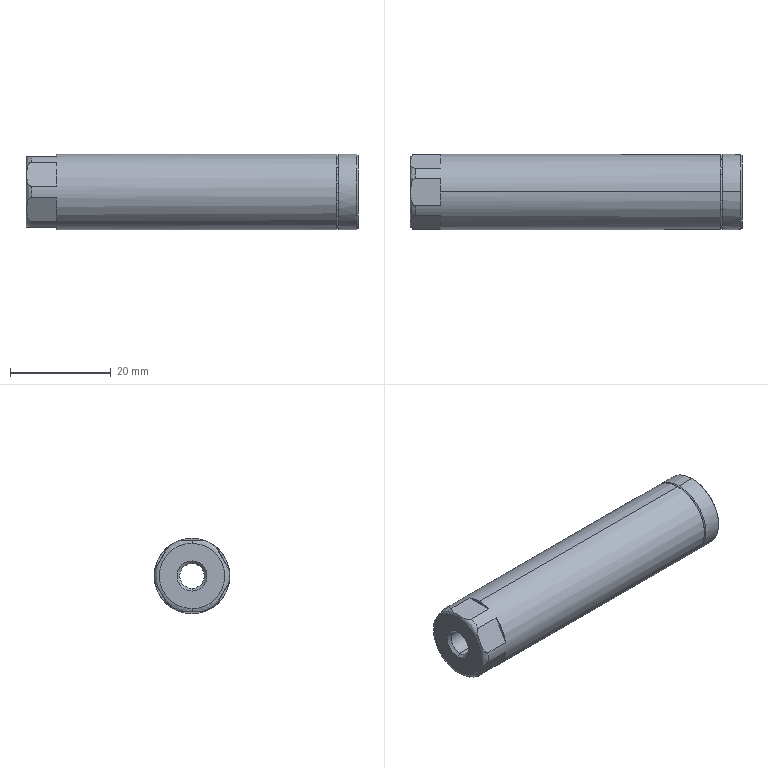Part | SolidWorks | features BaseBody 1 | 1 solid | 34 faces | box 66 x 15 x 15 mm | volume 8114 mm3 | plane 14 | cone 10 | cylinder 8 | spline 2 | commonest cylinder face diameters 15 x4 4.917 x2 8.5 x2
STEP:
#1=CARTESIAN_POINT('',(1.,-2.693,7.));
#2=VERTEX_POINT('',#1);
#3=CARTESIAN_POINT('',(0.134,0.,7.));
#4=VERTEX_POINT('',#3);
#5=CARTESIAN_POINT('',(1.,-2.693,7.));
#6=CARTESIAN_POINT('',(0.9357,-2.693,7.));
#7=CARTESIAN_POINT('',(0.8731,-2.675,7.));
#8=CARTESIAN_POINT('',(0.7611,-2.616,7.));
#9=CARTESIAN_POINT('',(0.7108,-2.575,7.));
#10=CARTESIAN_POINT('',(0.5795,-2.438,7.));
#11=CARTESIAN_POINT('',(0.5135,-2.327,7.));
#12=CARTESIAN_POINT('',(0.4066,-2.1,7.));
#13=CARTESIAN_POINT('',(0.3648,-1.98,7.));
#14=CARTESIAN_POINT('',(0.2958,-1.738,7.));
#15=CARTESIAN_POINT('',(0.2688,-1.616,7.));
#16=CARTESIAN_POINT('',(0.2018,-1.247,7.));
#17=CARTESIAN_POINT('',(0.1754,-0.9993,7.));
#18=CARTESIAN_POINT('',(0.1414,-0.5011,7.));
#19=CARTESIAN_POINT('',(0.134,-0.2503,7.));
#20=CARTESIAN_POINT('',(0.134,0.,7.));
#21=B_SPLINE_CURVE_WITH_KNOTS('',3,(#5,#6,#7,#8,#9,#10,#11,#12,#13,#14,#15,#16,#17,#18,#19,#20),.UNSPECIFIED.,.F.,.F.,(4,2,2,2,2,2,2,4),(0.,0.0001898,0.0003795,0.0007591,0.001139,0.001518,0.002277,0.003036),.UNSPECIFIED.);
#22=EDGE_CURVE('',#2,#4,#21,.T.);
#23=ORIENTED_EDGE('',*,*,#22,.T.);
#24=CARTESIAN_POINT('',(0.,0.,6.5));
#25=VERTEX_POINT('',#24);
#26=CARTESIAN_POINT('',(1.,0.,6.5));
#27=DIRECTION('',(0.,-1.,0.));
#28=DIRECTION('',(0.,0.,1.));
#29=AXIS2_PLACEMENT_3D('',#26,#27,#28);
#30=CIRCLE('',#29,1.);
#31=EDGE_CURVE('',#4,#25,#30,.T.);
#32=ORIENTED_EDGE('',*,*,#31,.T.);
#33=CARTESIAN_POINT('',(0.,0.,-6.5));
#34=VERTEX_POINT('',#33);
#35=CARTESIAN_POINT('',(0.,0.,6.5));
#36=CARTESIAN_POINT('',(0.,-13.,6.5));
#37=CARTESIAN_POINT('',(0.,-13.,-6.5));
#38=CARTESIAN_POINT('',(0.,0.,-6.5));
#39=(BOUNDED_CURVE()B_SPLINE_CURVE(3,(#35,#36,#37,#38),.UNSPECIFIED.,.F.,.F.)B_SPLINE_CURVE_WITH_KNOTS((4,4),(0.5,1.),.UNSPECIFIED.)CURVE()GEOMETRIC_REPRESENTATION_ITEM()RATIONAL_B_SPLINE_CURVE((1.,0.3333,0.3333,1.))REPRESENTATION_ITEM(''));
#40=EDGE_CURVE('',#25,#34,#39,.T.);
#41=ORIENTED_EDGE('',*,*,#40,.T.);
#42=CARTESIAN_POINT('',(0.134,0.,-7.));
#43=VERTEX_POINT('',#42);
#44=CARTESIAN_POINT('',(1.,0.,-6.5));
#45=DIRECTION('',(0.,1.,0.));
#46=DIRECTION('',(0.,0.,-1.));
#47=AXIS2_PLACEMENT_3D('',#44,#45,#46);
#48=CIRCLE('',#47,1.);
#49=EDGE_CURVE('',#43,#34,#48,.T.);
#50=ORIENTED_EDGE('',*,*,#49,.F.);
#51=CARTESIAN_POINT('',(1.,-2.693,-7.));
#52=VERTEX_POINT('',#51);
#53=CARTESIAN_POINT('',(0.134,0.,-7.));
#54=CARTESIAN_POINT('',(0.134,-0.2506,-7.));
#55=CARTESIAN_POINT('',(0.1413,-0.5008,-7.));
#56=CARTESIAN_POINT('',(0.1755,-0.9999,-7.));
#57=CARTESIAN_POINT('',(0.2019,-1.249,-7.));
#58=CARTESIAN_POINT('',(0.2924,-1.744,-7.));
#59=CARTESIAN_POINT('',(0.3546,-1.991,-7.));
#60=CARTESIAN_POINT('',(0.515,-2.33,-7.));
#61=CARTESIAN_POINT('',(0.5805,-2.44,-7.));
#62=CARTESIAN_POINT('',(0.7127,-2.576,-7.));
#63=CARTESIAN_POINT('',(0.7616,-2.616,-7.));
#64=CARTESIAN_POINT('',(0.8736,-2.675,-7.));
#65=CARTESIAN_POINT('',(0.9361,-2.693,-7.));
#66=CARTESIAN_POINT('',(1.,-2.693,-7.));
#67=B_SPLINE_CURVE_WITH_KNOTS('',3,(#53,#54,#55,#56,#57,#58,#59,#60,#61,#62,#63,#64,#65,#66),.UNSPECIFIED.,.F.,.F.,(4,2,2,2,2,2,4),(0.003036,0.003796,0.004556,0.005316,0.005696,0.005886,0.006076),.UNSPECIFIED.);
#68=EDGE_CURVE('',#43,#52,#67,.T.);
#69=ORIENTED_EDGE('',*,*,#68,.T.);
#70=CARTESIAN_POINT('',(1.,-4.716,-5.832));
#71=VERTEX_POINT('',#70);
#72=CARTESIAN_POINT('',(1.,0.,0.));
#73=DIRECTION('',(1.,0.,0.));
#74=DIRECTION('',(0.,0.,1.));
#75=AXIS2_PLACEMENT_3D('',#72,#73,#74);
#76=CIRCLE('',#75,7.5);
#77=EDGE_CURVE('',#71,#52,#76,.T.);
#78=ORIENTED_EDGE('',*,*,#77,.F.);
#79=CARTESIAN_POINT('',(1.,-7.408,-1.168));
#80=VERTEX_POINT('',#79);
#81=CARTESIAN_POINT('',(1.,-4.716,-5.832));
#82=CARTESIAN_POINT('',(0.9356,-4.716,-5.832));
#83=CARTESIAN_POINT('',(0.873,-4.725,-5.816));
#84=CARTESIAN_POINT('',(0.7609,-4.754,-5.765));
#85=CARTESIAN_POINT('',(0.7107,-4.775,-5.73));
#86=CARTESIAN_POINT('',(0.5793,-4.843,-5.611));
#87=CARTESIAN_POINT('',(0.5133,-4.899,-5.515));
#88=CARTESIAN_POINT('',(0.4064,-5.012,-5.318));
#89=CARTESIAN_POINT('',(0.3646,-5.072,-5.214));
#90=CARTESIAN_POINT('',(0.2956,-5.194,-5.004));
#91=CARTESIAN_POINT('',(0.2686,-5.255,-4.898));
#92=CARTESIAN_POINT('',(0.2016,-5.439,-4.579));
#93=CARTESIAN_POINT('',(0.1753,-5.563,-4.364));
#94=CARTESIAN_POINT('',(0.1413,-5.812,-3.933));
#95=CARTESIAN_POINT('',(0.1339,-5.938,-3.715));
#96=CARTESIAN_POINT('',(0.134,-6.188,-3.282));
#97=CARTESIAN_POINT('',(0.1414,-6.313,-3.065));
#98=CARTESIAN_POINT('',(0.1756,-6.563,-2.633));
#99=CARTESIAN_POINT('',(0.2021,-6.687,-2.417));
#100=CARTESIAN_POINT('',(0.2926,-6.935,-1.989));
#101=CARTESIAN_POINT('',(0.3548,-7.058,-1.776));
#102=CARTESIAN_POINT('',(0.5151,-7.227,-1.482));
#103=CARTESIAN_POINT('',(0.5807,-7.282,-1.387));
#104=CARTESIAN_POINT('',(0.7128,-7.35,-1.269));
#105=CARTESIAN_POINT('',(0.7617,-7.37,-1.234));
#106=CARTESIAN_POINT('',(0.8737,-7.4,-1.183));
#107=CARTESIAN_POINT('',(0.9361,-7.408,-1.168));
#108=CARTESIAN_POINT('',(1.,-7.408,-1.168));
#109=B_SPLINE_CURVE_WITH_KNOTS('',3,(#81,#82,#83,#84,#85,#86,#87,#88,#89,#90,#91,#92,#93,#94,#95,#96,#97,#98,#99,#100,#101,#102,#103,#104,#105,#106,#107,#108),.UNSPECIFIED.,.F.,.F.,(4,2,2,2,2,2,2,2,2,2,2,2,2,4),(0.,0.0001899,0.0003798,0.0007595,0.001139,0.001519,0.002279,0.003038,0.003798,0.004557,0.005317,0.005697,0.005887,0.006076),.UNSPECIFIED.);
#110=EDGE_CURVE('',#71,#80,#109,.T.);
#111=ORIENTED_EDGE('',*,*,#110,.T.);
#112=CARTESIAN_POINT('',(1.,-7.408,1.168));
#113=VERTEX_POINT('',#112);
#114=CARTESIAN_POINT('',(1.,0.,0.));
#115=DIRECTION('',(1.,0.,0.));
#116=DIRECTION('',(0.,0.,1.));
#117=AXIS2_PLACEMENT_3D('',#114,#115,#116);
#118=CIRCLE('',#117,7.5);
#119=EDGE_CURVE('',#113,#80,#118,.T.);
#120=ORIENTED_EDGE('',*,*,#119,.F.);
#121=CARTESIAN_POINT('',(1.,-4.716,5.832));
#122=VERTEX_POINT('',#121);
#123=CARTESIAN_POINT('',(1.,-7.408,1.168));
#124=CARTESIAN_POINT('',(0.9356,-7.408,1.168));
#125=CARTESIAN_POINT('',(0.873,-7.4,1.184));
#126=CARTESIAN_POINT('',(0.7609,-7.37,1.235));
#127=CARTESIAN_POINT('',(0.7107,-7.35,1.27));
#128=CARTESIAN_POINT('',(0.5793,-7.281,1.389));
#129=CARTESIAN_POINT('',(0.5133,-7.226,1.485));
#130=CARTESIAN_POINT('',(0.4064,-7.112,1.682));
#131=CARTESIAN_POINT('',(0.3646,-7.052,1.786));
#132=CARTESIAN_POINT('',(0.2956,-6.931,1.996));
#133=CARTESIAN_POINT('',(0.2686,-6.87,2.102));
#134=CARTESIAN_POINT('',(0.2016,-6.685,2.421));
#135=CARTESIAN_POINT('',(0.1753,-6.561,2.636));
#136=CARTESIAN_POINT('',(0.1413,-6.312,3.067));
#137=CARTESIAN_POINT('',(0.1339,-6.187,3.285));
#138=CARTESIAN_POINT('',(0.134,-5.936,3.718));
#139=CARTESIAN_POINT('',(0.1414,-5.811,3.935));
#140=CARTESIAN_POINT('',(0.1756,-5.562,4.367));
#141=CARTESIAN_POINT('',(0.2021,-5.437,4.583));
#142=CARTESIAN_POINT('',(0.2926,-5.19,5.011));
#143=CARTESIAN_POINT('',(0.3548,-5.067,5.224));
#144=CARTESIAN_POINT('',(0.5151,-4.897,5.518));
#145=CARTESIAN_POINT('',(0.5807,-4.842,5.613));
#146=CARTESIAN_POINT('',(0.7128,-4.774,5.731));
#147=CARTESIAN_POINT('',(0.7617,-4.754,5.766));
#148=CARTESIAN_POINT('',(0.8737,-4.725,5.817));
#149=CARTESIAN_POINT('',(0.9361,-4.716,5.832));
#150=CARTESIAN_POINT('',(1.,-4.716,5.832));
#151=B_SPLINE_CURVE_WITH_KNOTS('',3,(#123,#124,#125,#126,#127,#128,#129,#130,#131,#132,#133,#134,#135,#136,#137,#138,#139,#140,#141,#142,#143,#144,#145,#146,#147,#148,#149,#150),.UNSPECIFIED.,.F.,.F.,(4,2,2,2,2,2,2,2,2,2,2,2,2,4),(0.,0.0001899,0.0003798,0.0007595,0.001139,0.001519,0.002279,0.003038,0.003798,0.004557,0.005317,0.005697,0.005887,0.006076),.UNSPECIFIED.);
#152=EDGE_CURVE('',#113,#122,#151,.T.);
#153=ORIENTED_EDGE('',*,*,#152,.T.);
#154=CARTESIAN_POINT('',(1.,0.,0.));
#155=DIRECTION('',(1.,0.,0.));
#156=DIRECTION('',(0.,0.,1.));
#157=AXIS2_PLACEMENT_3D('',#154,#155,#156);
#158=CIRCLE('',#157,7.5);
#159=EDGE_CURVE('',#2,#122,#158,.T.);
#160=ORIENTED_EDGE('',*,*,#159,.F.);
#161=EDGE_LOOP('',(#23,#32,#41,#50,#69,#78,#111,#120,#153,#160));
#162=FACE_OUTER_BOUND('',#161,.T.);
#163=CARTESIAN_POINT('',(1.,0.,7.5));
#164=CARTESIAN_POINT('',(1.,-15.,7.5));
#165=CARTESIAN_POINT('',(1.,-15.,-7.5));
#166=CARTESIAN_POINT('',(1.,0.,-7.5));
#167=CARTESIAN_POINT('',(0.4142,0.,7.5));
#168=CARTESIAN_POINT('',(0.4142,-15.,7.5));
#169=CARTESIAN_POINT('',(0.4142,-15.,-7.5));
#170=CARTESIAN_POINT('',(0.4142,0.,-7.5));
#171=CARTESIAN_POINT('',(0.,0.,7.086));
#172=CARTESIAN_POINT('',(0.,-14.172,7.086));
#173=CARTESIAN_POINT('',(0.,-14.172,-7.086));
#174=CARTESIAN_POINT('',(0.,0.,-7.086));
#175=CARTESIAN_POINT('',(0.,0.,6.5));
#176=CARTESIAN_POINT('',(0.,-13.,6.5));
#177=CARTESIAN_POINT('',(0.,-13.,-6.5));
#178=CARTESIAN_POINT('',(0.,0.,-6.5));
#179=(BOUNDED_SURFACE()B_SPLINE_SURFACE(3,3,((#163,#164,#165,#166),(#167,#168,#169,#170),(#171,#172,#173,#174),(#175,#176,#177,#178)),.UNSPECIFIED.,.F.,.F.,.F.)B_SPLINE_SURFACE_WITH_KNOTS((4,4),(4,4),(0.,1.),(0.,1.),.UNSPECIFIED.)GEOMETRIC_REPRESENTATION_ITEM()RATIONAL_B_SPLINE_SURFACE(((1.,0.3333,0.3333,1.),(0.8047,0.2682,0.2682,0.8047),(0.8047,0.2682,0.2682,0.8047),(1.,0.3333,0.3333,1.)))REPRESENTATION_ITEM('')SURFACE());
#180=ADVANCED_FACE('',(#162),#179,.T.);
#181=CARTESIAN_POINT('',(61.8,0.,7.5));
#182=VERTEX_POINT('',#181);
#183=CARTESIAN_POINT('',(61.8,0.,-7.5));
#184=VERTEX_POINT('',#183);
#185=CARTESIAN_POINT('',(61.8,0.,0.));
#186=DIRECTION('',(-1.,0.,0.));
#187=DIRECTION('',(0.,0.,1.));
#188=AXIS2_PLACEMENT_3D('',#185,#186,#187);
#189=CIRCLE('',#188,7.5);
#190=EDGE_CURVE('',#182,#184,#189,.T.);
#191=ORIENTED_EDGE('',*,*,#190,.T.);
#192=CARTESIAN_POINT('',(6.,0.,-7.5));
#193=VERTEX_POINT('',#192);
#194=CARTESIAN_POINT('',(66.,0.,-7.5));
#195=DIRECTION('',(-1.,0.,0.));
#196=VECTOR('',#195,1000.);
#197=LINE('',#194,#196);
#198=EDGE_CURVE('',#184,#193,#197,.T.);
#199=ORIENTED_EDGE('',*,*,#198,.T.);
#200=CARTESIAN_POINT('',(6.,2.693,-7.));
#201=VERTEX_POINT('',#200);
#202=CARTESIAN_POINT('',(6.,0.,0.));
#203=DIRECTION('',(1.,0.,0.));
#204=DIRECTION('',(0.,0.,1.));
#205=AXIS2_PLACEMENT_3D('',#202,#203,#204);
#206=CIRCLE('',#205,7.5);
#207=EDGE_CURVE('',#193,#201,#206,.T.);
#208=ORIENTED_EDGE('',*,*,#207,.T.);
#209=CARTESIAN_POINT('',(1.,2.693,-7.));
#210=VERTEX_POINT('',#209);
#211=CARTESIAN_POINT('',(66.,2.693,-7.));
#212=DIRECTION('',(-1.,0.,0.));
#213=VECTOR('',#212,1000.);
#214=LINE('',#211,#213);
#215=EDGE_CURVE('',#201,#210,#214,.T.);
#216=ORIENTED_EDGE('',*,*,#215,.T.);
#217=CARTESIAN_POINT('',(1.,4.716,-5.832));
#218=VERTEX_POINT('',#217);
#219=CARTESIAN_POINT('',(1.,0.,0.));
#220=DIRECTION('',(1.,0.,0.));
#221=DIRECTION('',(0.,0.,1.));
#222=AXIS2_PLACEMENT_3D('',#219,#220,#221);
#223=CIRCLE('',#222,7.5);
#224=EDGE_CURVE('',#210,#218,#223,.T.);
#225=ORIENTED_EDGE('',*,*,#224,.T.);
#226=CARTESIAN_POINT('',(6.,4.716,-5.832));
#227=VERTEX_POINT('',#226);
#228=CARTESIAN_POINT('',(66.,4.716,-5.832));
#229=DIRECTION('',(1.,0.,0.));
#230=VECTOR('',#229,1000.);
#231=LINE('',#228,#230);
#232=EDGE_CURVE('',#218,#227,#231,.T.);
#233=ORIENTED_EDGE('',*,*,#232,.T.);
#234=CARTESIAN_POINT('',(6.,7.408,-1.168));
#235=VERTEX_POINT('',#234);
#236=CARTESIAN_POINT('',(6.,0.,0.));
#237=DIRECTION('',(1.,0.,0.));
#238=DIRECTION('',(0.,0.,1.));
#239=AXIS2_PLACEMENT_3D('',#236,#237,#238);
#240=CIRCLE('',#239,7.5);
#241=EDGE_CURVE('',#227,#235,#240,.T.);
#242=ORIENTED_EDGE('',*,*,#241,.T.);
#243=CARTESIAN_POINT('',(1.,7.408,-1.168));
#244=VERTEX_POINT('',#243);
#245=CARTESIAN_POINT('',(66.,7.408,-1.168));
#246=DIRECTION('',(-1.,0.,0.));
#247=VECTOR('',#246,1000.);
#248=LINE('',#245,#247);
#249=EDGE_CURVE('',#235,#244,#248,.T.);
#250=ORIENTED_EDGE('',*,*,#249,.T.);
#251=CARTESIAN_POINT('',(1.,7.408,1.168));
#252=VERTEX_POINT('',#251);
#253=CARTESIAN_POINT('',(1.,0.,0.));
#254=DIRECTION('',(1.,0.,0.));
#255=DIRECTION('',(0.,0.,1.));
#256=AXIS2_PLACEMENT_3D('',#253,#254,#255);
#257=CIRCLE('',#256,7.5);
#258=EDGE_CURVE('',#244,#252,#257,.T.);
#259=ORIENTED_EDGE('',*,*,#258,.T.);
#260=CARTESIAN_POINT('',(6.,7.408,1.168));
#261=VERTEX_POINT('',#260);
#262=CARTESIAN_POINT('',(66.,7.408,1.168));
#263=DIRECTION('',(1.,0.,0.));
#264=VECTOR('',#263,1000.);
#265=LINE('',#262,#264);
#266=EDGE_CURVE('',#252,#261,#265,.T.);
#267=ORIENTED_EDGE('',*,*,#266,.T.);
#268=CARTESIAN_POINT('',(6.,4.716,5.832));
#269=VERTEX_POINT('',#268);
#270=CARTESIAN_POINT('',(6.,0.,0.));
#271=DIRECTION('',(1.,0.,0.));
#272=DIRECTION('',(0.,0.,1.));
#273=AXIS2_PLACEMENT_3D('',#270,#271,#272);
#274=CIRCLE('',#273,7.5);
#275=EDGE_CURVE('',#261,#269,#274,.T.);
#276=ORIENTED_EDGE('',*,*,#275,.T.);
#277=CARTESIAN_POINT('',(1.,4.716,5.832));
#278=VERTEX_POINT('',#277);
#279=CARTESIAN_POINT('',(66.,4.716,5.832));
#280=DIRECTION('',(-1.,0.,0.));
#281=VECTOR('',#280,1000.);
#282=LINE('',#279,#281);
#283=EDGE_CURVE('',#269,#278,#282,.T.);
#284=ORIENTED_EDGE('',*,*,#283,.T.);
#285=CARTESIAN_POINT('',(1.,2.693,7.));
#286=VERTEX_POINT('',#285);
#287=CARTESIAN_POINT('',(1.,0.,0.));
#288=DIRECTION('',(1.,0.,0.));
#289=DIRECTION('',(0.,0.,1.));
#290=AXIS2_PLACEMENT_3D('',#287,#288,#289);
#291=CIRCLE('',#290,7.5);
#292=EDGE_CURVE('',#278,#286,#291,.T.);
#293=ORIENTED_EDGE('',*,*,#292,.T.);
#294=CARTESIAN_POINT('',(6.,2.693,7.));
#295=VERTEX_POINT('',#294);
#296=CARTESIAN_POINT('',(66.,2.693,7.));
#297=DIRECTION('',(1.,0.,0.));
#298=VECTOR('',#297,1000.);
#299=LINE('',#296,#298);
#300=EDGE_CURVE('',#286,#295,#299,.T.);
#301=ORIENTED_EDGE('',*,*,#300,.T.);
#302=CARTESIAN_POINT('',(6.,0.,7.5));
#303=VERTEX_POINT('',#302);
#304=CARTESIAN_POINT('',(6.,0.,0.));
#305=DIRECTION('',(1.,0.,0.));
#306=DIRECTION('',(0.,0.,1.));
#307=AXIS2_PLACEMENT_3D('',#304,#305,#306);
#308=CIRCLE('',#307,7.5);
#309=EDGE_CURVE('',#295,#303,#308,.T.);
#310=ORIENTED_EDGE('',*,*,#309,.T.);
#311=CARTESIAN_POINT('',(66.,0.,7.5));
#312=DIRECTION('',(-1.,0.,0.));
#313=VECTOR('',#312,1000.);
#314=LINE('',#311,#313);
#315=EDGE_CURVE('',#182,#303,#314,.T.);
#316=ORIENTED_EDGE('',*,*,#315,.F.);
#317=EDGE_LOOP('',(#191,#199,#208,#216,#225,#233,#242,#250,#259,#267,#276,#284,#293,#301,#310,#316));
#318=FACE_OUTER_BOUND('',#317,.T.);
#319=CARTESIAN_POINT('',(66.,0.,0.));
#320=DIRECTION('',(-1.,0.,0.));
#321=DIRECTION('',(0.,0.,1.));
#322=AXIS2_PLACEMENT_3D('',#319,#320,#321);
#323=CYLINDRICAL_SURFACE('',#322,7.5);
#324=ADVANCED_FACE('',(#318),#323,.T.);
#325=CARTESIAN_POINT('',(62.,7.3,0.));
#326=VERTEX_POINT('',#325);
#327=CARTESIAN_POINT('',(62.,0.,-7.3));
#328=VERTEX_POINT('',#327);
#329=CARTESIAN_POINT('',(62.,0.,0.));
#330=DIRECTION('',(-1.,0.,0.));
#331=DIRECTION('',(0.,0.,1.));
#332=AXIS2_PLACEMENT_3D('',#329,#330,#331);
#333=CIRCLE('',#332,7.3);
#334=EDGE_CURVE('',#326,#328,#333,.T.);
#335=ORIENTED_EDGE('',*,*,#334,.T.);
#336=CARTESIAN_POINT('',(61.8,0.,-7.5));
#337=DIRECTION('',(-0.7071,0.,-0.7071));
#338=VECTOR('',#337,1000.);
#339=LINE('',#336,#338);
#340=EDGE_CURVE('',#328,#184,#339,.T.);
#341=ORIENTED_EDGE('',*,*,#340,.T.);
#342=ORIENTED_EDGE('',*,*,#190,.F.);
#343=CARTESIAN_POINT('',(62.,0.,7.3));
#344=VERTEX_POINT('',#343);
#345=CARTESIAN_POINT('',(61.8,0.,7.5));
#346=DIRECTION('',(-0.7071,0.,0.7071));
#347=VECTOR('',#346,1000.);
#348=LINE('',#345,#347);
#349=EDGE_CURVE('',#344,#182,#348,.T.);
#350=ORIENTED_EDGE('',*,*,#349,.F.);
#351=CARTESIAN_POINT('',(62.,0.,0.));
#352=DIRECTION('',(-1.,0.,0.));
#353=DIRECTION('',(0.,0.,1.));
#354=AXIS2_PLACEMENT_3D('',#351,#352,#353);
#355=CIRCLE('',#354,7.3);
#356=EDGE_CURVE('',#344,#326,#355,.T.);
#357=ORIENTED_EDGE('',*,*,#356,.T.);
#358=EDGE_LOOP('',(#335,#341,#342,#350,#357));
#359=FACE_OUTER_BOUND('',#358,.T.);
#360=CARTESIAN_POINT('',(61.8,0.,0.));
#361=DIRECTION('',(-1.,0.,0.));
#362=DIRECTION('',(0.,0.,1.));
#363=AXIS2_PLACEMENT_3D('',#360,#361,#362);
#364=CONICAL_SURFACE('',#363,7.5,0.7854);
#365=ADVANCED_FACE('',(#359),#364,.T.);
#366=CARTESIAN_POINT('',(62.,-7.3,0.));
#367=VERTEX_POINT('',#366);
#368=CARTESIAN_POINT('',(62.,0.,0.));
#369=DIRECTION('',(-1.,0.,0.));
#370=DIRECTION('',(0.,0.,1.));
#371=AXIS2_PLACEMENT_3D('',#368,#369,#370);
#372=CIRCLE('',#371,7.3);
#373=EDGE_CURVE('',#367,#344,#372,.T.);
#374=ORIENTED_EDGE('',*,*,#373,.F.);
#375=CARTESIAN_POINT('',(62.2,-7.5,0.));
#376=VERTEX_POINT('',#375);
#377=CARTESIAN_POINT('',(62.2,-7.5,0.));
#378=DIRECTION('',(0.7071,-0.7071,0.));
#379=VECTOR('',#378,1000.);
#380=LINE('',#377,#379);
#381=EDGE_CURVE('',#367,#376,#380,.T.);
#382=ORIENTED_EDGE('',*,*,#381,.T.);
#383=CARTESIAN_POINT('',(62.2,0.,7.5));
#384=VERTEX_POINT('',#383);
#385=CARTESIAN_POINT('',(62.2,0.,0.));
#386=DIRECTION('',(-1.,0.,0.));
#387=DIRECTION('',(0.,0.,-1.));
#388=AXIS2_PLACEMENT_3D('',#385,#386,#387);
#389=CIRCLE('',#388,7.5);
#390=EDGE_CURVE('',#376,#384,#389,.T.);
#391=ORIENTED_EDGE('',*,*,#390,.T.);
#392=CARTESIAN_POINT('',(62.2,7.5,0.));
#393=VERTEX_POINT('',#392);
#394=CARTESIAN_POINT('',(62.2,0.,0.));
#395=DIRECTION('',(-1.,0.,0.));
#396=DIRECTION('',(0.,0.,-1.));
#397=AXIS2_PLACEMENT_3D('',#394,#395,#396);
#398=CIRCLE('',#397,7.5);
#399=EDGE_CURVE('',#384,#393,#398,.T.);
#400=ORIENTED_EDGE('',*,*,#399,.T.);
#401=CARTESIAN_POINT('',(62.2,7.5,0.));
#402=DIRECTION('',(0.7071,0.7071,0.));
#403=VECTOR('',#402,1000.);
#404=LINE('',#401,#403);
#405=EDGE_CURVE('',#326,#393,#404,.T.);
#406=ORIENTED_EDGE('',*,*,#405,.F.);
#407=ORIENTED_EDGE('',*,*,#356,.F.);
#408=EDGE_LOOP('',(#374,#382,#391,#400,#406,#407));
#409=FACE_OUTER_BOUND('',#408,.T.);
#410=CARTESIAN_POINT('',(62.2,0.,0.));
#411=DIRECTION('',(1.,0.,0.));
#412=DIRECTION('',(0.,1.,0.));
#413=AXIS2_PLACEMENT_3D('',#410,#411,#412);
#414=CONICAL_SURFACE('',#413,7.5,0.7854);
#415=ADVANCED_FACE('',(#409),#414,.T.);
#416=CARTESIAN_POINT('',(65.8,0.,7.5));
#417=VERTEX_POINT('',#416);
#418=CARTESIAN_POINT('',(65.8,0.,-7.5));
#419=VERTEX_POINT('',#418);
#420=CARTESIAN_POINT('',(65.8,0.,0.));
#421=DIRECTION('',(-1.,0.,0.));
#422=DIRECTION('',(0.,0.,1.));
#423=AXIS2_PLACEMENT_3D('',#420,#421,#422);
#424=CIRCLE('',#423,7.5);
#425=EDGE_CURVE('',#417,#419,#424,.T.);
#426=ORIENTED_EDGE('',*,*,#425,.T.);
#427=CARTESIAN_POINT('',(62.2,0.,-7.5));
#428=VERTEX_POINT('',#427);
#429=CARTESIAN_POINT('',(66.,0.,-7.5));
#430=DIRECTION('',(-1.,0.,0.));
#431=VECTOR('',#430,1000.);
#432=LINE('',#429,#431);
#433=EDGE_CURVE('',#419,#428,#432,.T.);
#434=ORIENTED_EDGE('',*,*,#433,.T.);
#435=CARTESIAN_POINT('',(62.2,0.,0.));
#436=DIRECTION('',(-1.,0.,0.));
#437=DIRECTION('',(0.,0.,-1.));
#438=AXIS2_PLACEMENT_3D('',#435,#436,#437);
#439=CIRCLE('',#438,7.5);
#440=EDGE_CURVE('',#393,#428,#439,.T.);
#441=ORIENTED_EDGE('',*,*,#440,.F.);
#442=ORIENTED_EDGE('',*,*,#399,.F.);
#443=CARTESIAN_POINT('',(66.,0.,7.5));
#444=DIRECTION('',(-1.,0.,0.));
#445=VECTOR('',#444,1000.);
#446=LINE('',#443,#445);
#447=EDGE_CURVE('',#417,#384,#446,.T.);
#448=ORIENTED_EDGE('',*,*,#447,.F.);
#449=EDGE_LOOP('',(#426,#434,#441,#442,#448));
#450=FACE_OUTER_BOUND('',#449,.T.);
#451=CARTESIAN_POINT('',(66.,0.,0.));
#452=DIRECTION('',(-1.,0.,0.));
#453=DIRECTION('',(0.,0.,1.));
#454=AXIS2_PLACEMENT_3D('',#451,#452,#453);
#455=CYLINDRICAL_SURFACE('',#454,7.5);
#456=ADVANCED_FACE('',(#450),#455,.T.);
#457=CARTESIAN_POINT('',(0.5415,0.,-2.458));
#458=VERTEX_POINT('',#457);
#459=CARTESIAN_POINT('',(0.5415,0.,2.458));
#460=VERTEX_POINT('',#459);
#461=CARTESIAN_POINT('',(0.5415,0.,0.));
#462=DIRECTION('',(-1.,0.,0.));
#463=DIRECTION('',(0.,0.,1.));
#464=AXIS2_PLACEMENT_3D('',#461,#462,#463);
#465=CIRCLE('',#464,2.458);
#466=EDGE_CURVE('',#458,#460,#465,.T.);
#467=ORIENTED_EDGE('',*,*,#466,.F.);
#468=CARTESIAN_POINT('',(0.,0.,-3.));
#469=VERTEX_POINT('',#468);
#470=CARTESIAN_POINT('',(0.,0.,-3.));
#471=DIRECTION('',(-0.7071,0.,-0.7071));
#472=VECTOR('',#471,1000.);
#473=LINE('',#470,#472);
#474=EDGE_CURVE('',#458,#469,#473,.T.);
#475=ORIENTED_EDGE('',*,*,#474,.T.);
#476=CARTESIAN_POINT('',(0.,0.,3.));
#477=VERTEX_POINT('',#476);
#478=CARTESIAN_POINT('',(0.,0.,0.));
#479=DIRECTION('',(1.,0.,0.));
#480=DIRECTION('',(0.,0.,1.));
#481=AXIS2_PLACEMENT_3D('',#478,#479,#480);
#482=CIRCLE('',#481,3.);
#483=EDGE_CURVE('',#477,#469,#482,.T.);
#484=ORIENTED_EDGE('',*,*,#483,.F.);
#485=CARTESIAN_POINT('',(0.,0.,3.));
#486=DIRECTION('',(-0.7071,0.,0.7071));
#487=VECTOR('',#486,1000.);
#488=LINE('',#485,#487);
#489=EDGE_CURVE('',#460,#477,#488,.T.);
#490=ORIENTED_EDGE('',*,*,#489,.F.);
#491=EDGE_LOOP('',(#467,#475,#484,#490));
#492=FACE_OUTER_BOUND('',#491,.T.);
#493=CARTESIAN_POINT('',(0.,0.,0.));
#494=DIRECTION('',(-1.,0.,0.));
#495=DIRECTION('',(0.,0.,1.));
#496=AXIS2_PLACEMENT_3D('',#493,#494,#495);
#497=CONICAL_SURFACE('',#496,3.,0.7854);
#498=ADVANCED_FACE('',(#492),#497,.F.);
#499=CARTESIAN_POINT('',(66.,0.,7.3));
#500=VERTEX_POINT('',#499);
#501=CARTESIAN_POINT('',(66.,0.,-7.3));
#502=VERTEX_POINT('',#501);
#503=CARTESIAN_POINT('',(66.,0.,0.));
#504=DIRECTION('',(-1.,0.,0.));
#505=DIRECTION('',(0.,0.,1.));
#506=AXIS2_PLACEMENT_3D('',#503,#504,#505);
#507=CIRCLE('',#506,7.3);
#508=EDGE_CURVE('',#500,#502,#507,.T.);
#509=ORIENTED_EDGE('',*,*,#508,.T.);
#510=CARTESIAN_POINT('',(65.8,0.,-7.5));
#511=DIRECTION('',(-0.7071,0.,-0.7071));
#512=VECTOR('',#511,1000.);
#513=LINE('',#510,#512);
#514=EDGE_CURVE('',#502,#419,#513,.T.);
#515=ORIENTED_EDGE('',*,*,#514,.T.);
#516=ORIENTED_EDGE('',*,*,#425,.F.);
#517=CARTESIAN_POINT('',(65.8,0.,7.5));
#518=DIRECTION('',(-0.7071,0.,0.7071));
#519=VECTOR('',#518,1000.);
#520=LINE('',#517,#519);
#521=EDGE_CURVE('',#500,#417,#520,.T.);
#522=ORIENTED_EDGE('',*,*,#521,.F.);
#523=EDGE_LOOP('',(#509,#515,#516,#522));
#524=FACE_OUTER_BOUND('',#523,.T.);
#525=CARTESIAN_POINT('',(65.8,0.,0.));
#526=DIRECTION('',(-1.,0.,0.));
#527=DIRECTION('',(0.,0.,1.));
#528=AXIS2_PLACEMENT_3D('',#525,#526,#527);
#529=CONICAL_SURFACE('',#528,7.5,0.7854);
#530=ADVANCED_FACE('',(#524),#529,.T.);
#531=CARTESIAN_POINT('',(6.208,0.,-2.458));
#532=VERTEX_POINT('',#531);
#533=CARTESIAN_POINT('',(6.208,0.,2.458));
#534=VERTEX_POINT('',#533);
#535=CARTESIAN_POINT('',(6.208,0.,0.));
#536=DIRECTION('',(-1.,0.,0.));
#537=DIRECTION('',(0.,0.,1.));
#538=AXIS2_PLACEMENT_3D('',#535,#536,#537);
#539=CIRCLE('',#538,2.458);
#540=EDGE_CURVE('',#532,#534,#539,.T.);
#541=ORIENTED_EDGE('',*,*,#540,.F.);
#542=CARTESIAN_POINT('',(66.,0.,-2.458));
#543=DIRECTION('',(-1.,0.,0.));
#544=VECTOR('',#543,1000.);
#545=LINE('',#542,#544);
#546=EDGE_CURVE('',#532,#458,#545,.T.);
#547=ORIENTED_EDGE('',*,*,#546,.T.);
#548=ORIENTED_EDGE('',*,*,#466,.T.);
#549=CARTESIAN_POINT('',(66.,0.,2.458));
#550=DIRECTION('',(-1.,0.,0.));
#551=VECTOR('',#550,1000.);
#552=LINE('',#549,#551);
#553=EDGE_CURVE('',#534,#460,#552,.T.);
#554=ORIENTED_EDGE('',*,*,#553,.F.);
#555=EDGE_LOOP('',(#541,#547,#548,#554));
#556=FACE_OUTER_BOUND('',#555,.T.);
#557=CARTESIAN_POINT('',(66.,0.,0.));
#558=DIRECTION('',(-1.,0.,0.));
#559=DIRECTION('',(0.,0.,1.));
#560=AXIS2_PLACEMENT_3D('',#557,#558,#559);
#561=CYLINDRICAL_SURFACE('',#560,2.458);
#562=ADVANCED_FACE('',(#556),#561,.F.);
#563=ORIENTED_EDGE('',*,*,#540,.T.);
#564=CARTESIAN_POINT('',(8.,0.,4.25));
#565=VERTEX_POINT('',#564);
#566=CARTESIAN_POINT('',(8.,0.,4.25));
#567=DIRECTION('',(0.7071,0.,0.7071));
#568=VECTOR('',#567,1000.);
#569=LINE('',#566,#568);
#570=EDGE_CURVE('',#534,#565,#569,.T.);
#571=ORIENTED_EDGE('',*,*,#570,.T.);
#572=CARTESIAN_POINT('',(8.,0.,-4.25));
#573=VERTEX_POINT('',#572);
#574=CARTESIAN_POINT('',(8.,0.,0.));
#575=DIRECTION('',(-1.,0.,0.));
#576=DIRECTION('',(0.,0.,-1.));
#577=AXIS2_PLACEMENT_3D('',#574,#575,#576);
#578=CIRCLE('',#577,4.25);
#579=EDGE_CURVE('',#573,#565,#578,.T.);
#580=ORIENTED_EDGE('',*,*,#579,.F.);
#581=CARTESIAN_POINT('',(8.,0.,-4.25));
#582=DIRECTION('',(0.7071,0.,-0.7071));
#583=VECTOR('',#582,1000.);
#584=LINE('',#581,#583);
#585=EDGE_CURVE('',#532,#573,#584,.T.);
#586=ORIENTED_EDGE('',*,*,#585,.F.);
#587=EDGE_LOOP('',(#563,#571,#580,#586));
#588=FACE_OUTER_BOUND('',#587,.T.);
#589=CARTESIAN_POINT('',(8.,0.,0.));
#590=DIRECTION('',(1.,0.,0.));
#591=DIRECTION('',(0.,0.,-1.));
#592=AXIS2_PLACEMENT_3D('',#589,#590,#591);
#593=CONICAL_SURFACE('',#592,4.25,0.7854);
#594=ADVANCED_FACE('',(#588),#593,.F.);
#595=CARTESIAN_POINT('',(66.,0.,-4.25));
#596=VERTEX_POINT('',#595);
#597=CARTESIAN_POINT('',(66.,0.,4.25));
#598=VERTEX_POINT('',#597);
#599=CARTESIAN_POINT('',(66.,0.,0.));
#600=DIRECTION('',(-1.,0.,0.));
#601=DIRECTION('',(0.,0.,1.));
#602=AXIS2_PLACEMENT_3D('',#599,#600,#601);
#603=CIRCLE('',#602,4.25);
#604=EDGE_CURVE('',#596,#598,#603,.T.);
#605=ORIENTED_EDGE('',*,*,#604,.F.);
#606=CARTESIAN_POINT('',(66.,0.,-4.25));
#607=DIRECTION('',(-1.,0.,0.));
#608=VECTOR('',#607,1000.);
#609=LINE('',#606,#608);
#610=EDGE_CURVE('',#596,#573,#609,.T.);
#611=ORIENTED_EDGE('',*,*,#610,.T.);
#612=ORIENTED_EDGE('',*,*,#579,.T.);
#613=CARTESIAN_POINT('',(66.,0.,4.25));
#614=DIRECTION('',(-1.,0.,0.));
#615=VECTOR('',#614,1000.);
#616=LINE('',#613,#615);
#617=EDGE_CURVE('',#598,#565,#616,.T.);
#618=ORIENTED_EDGE('',*,*,#617,.F.);
#619=EDGE_LOOP('',(#605,#611,#612,#618));
#620=FACE_OUTER_BOUND('',#619,.T.);
#621=CARTESIAN_POINT('',(66.,0.,0.));
#622=DIRECTION('',(-1.,0.,0.));
#623=DIRECTION('',(0.,0.,1.));
#624=AXIS2_PLACEMENT_3D('',#621,#622,#623);
#625=CYLINDRICAL_SURFACE('',#624,4.25);
#626=ADVANCED_FACE('',(#620),#625,.F.);
#627=ORIENTED_EDGE('',*,*,#198,.F.);
#628=CARTESIAN_POINT('',(61.8,0.,0.));
#629=DIRECTION('',(-1.,0.,0.));
#630=DIRECTION('',(0.,0.,1.));
#631=AXIS2_PLACEMENT_3D('',#628,#629,#630);
#632=CIRCLE('',#631,7.5);
#633=EDGE_CURVE('',#184,#182,#632,.T.);
#634=ORIENTED_EDGE('',*,*,#633,.T.);
#635=ORIENTED_EDGE('',*,*,#315,.T.);
#636=CARTESIAN_POINT('',(6.,-2.693,7.));
#637=VERTEX_POINT('',#636);
#638=CARTESIAN_POINT('',(6.,0.,0.));
#639=DIRECTION('',(1.,0.,0.));
#640=DIRECTION('',(0.,0.,1.));
#641=AXIS2_PLACEMENT_3D('',#638,#639,#640);
#642=CIRCLE('',#641,7.5);
#643=EDGE_CURVE('',#303,#637,#642,.T.);
#644=ORIENTED_EDGE('',*,*,#643,.T.);
#645=CARTESIAN_POINT('',(66.,-2.693,7.));
#646=DIRECTION('',(-1.,0.,0.));
#647=VECTOR('',#646,1000.);
#648=LINE('',#645,#647);
#649=EDGE_CURVE('',#637,#2,#648,.T.);
#650=ORIENTED_EDGE('',*,*,#649,.T.);
#651=ORIENTED_EDGE('',*,*,#159,.T.);
#652=CARTESIAN_POINT('',(6.,-4.716,5.832));
#653=VERTEX_POINT('',#652);
#654=CARTESIAN_POINT('',(66.,-4.716,5.832));
#655=DIRECTION('',(1.,0.,0.));
#656=VECTOR('',#655,1000.);
#657=LINE('',#654,#656);
#658=EDGE_CURVE('',#122,#653,#657,.T.);
#659=ORIENTED_EDGE('',*,*,#658,.T.);
#660=CARTESIAN_POINT('',(6.,-7.408,1.168));
#661=VERTEX_POINT('',#660);
#662=CARTESIAN_POINT('',(6.,0.,0.));
#663=DIRECTION('',(1.,0.,0.));
#664=DIRECTION('',(0.,0.,1.));
#665=AXIS2_PLACEMENT_3D('',#662,#663,#664);
#666=CIRCLE('',#665,7.5);
#667=EDGE_CURVE('',#653,#661,#666,.T.);
#668=ORIENTED_EDGE('',*,*,#667,.T.);
#669=CARTESIAN_POINT('',(66.,-7.408,1.168));
#670=DIRECTION('',(-1.,0.,0.));
#671=VECTOR('',#670,1000.);
#672=LINE('',#669,#671);
#673=EDGE_CURVE('',#661,#113,#672,.T.);
#674=ORIENTED_EDGE('',*,*,#673,.T.);
#675=ORIENTED_EDGE('',*,*,#119,.T.);
#676=CARTESIAN_POINT('',(6.,-7.408,-1.168));
#677=VERTEX_POINT('',#676);
#678=CARTESIAN_POINT('',(66.,-7.408,-1.168));
#679=DIRECTION('',(1.,0.,0.));
#680=VECTOR('',#679,1000.);
#681=LINE('',#678,#680);
#682=EDGE_CURVE('',#80,#677,#681,.T.);
#683=ORIENTED_EDGE('',*,*,#682,.T.);
#684=CARTESIAN_POINT('',(6.,-4.716,-5.832));
#685=VERTEX_POINT('',#684);
#686=CARTESIAN_POINT('',(6.,0.,0.));
#687=DIRECTION('',(1.,0.,0.));
#688=DIRECTION('',(0.,0.,1.));
#689=AXIS2_PLACEMENT_3D('',#686,#687,#688);
#690=CIRCLE('',#689,7.5);
#691=EDGE_CURVE('',#677,#685,#690,.T.);
#692=ORIENTED_EDGE('',*,*,#691,.T.);
#693=CARTESIAN_POINT('',(66.,-4.716,-5.832));
#694=DIRECTION('',(-1.,0.,0.));
#695=VECTOR('',#694,1000.);
#696=LINE('',#693,#695);
#697=EDGE_CURVE('',#685,#71,#696,.T.);
#698=ORIENTED_EDGE('',*,*,#697,.T.);
#699=ORIENTED_EDGE('',*,*,#77,.T.);
#700=CARTESIAN_POINT('',(6.,-2.693,-7.));
#701=VERTEX_POINT('',#700);
#702=CARTESIAN_POINT('',(66.,-2.693,-7.));
#703=DIRECTION('',(1.,0.,0.));
#704=VECTOR('',#703,1000.);
#705=LINE('',#702,#704);
#706=EDGE_CURVE('',#52,#701,#705,.T.);
#707=ORIENTED_EDGE('',*,*,#706,.T.);
#708=CARTESIAN_POINT('',(6.,0.,0.));
#709=DIRECTION('',(1.,0.,0.));
#710=DIRECTION('',(0.,0.,1.));
#711=AXIS2_PLACEMENT_3D('',#708,#709,#710);
#712=CIRCLE('',#711,7.5);
#713=EDGE_CURVE('',#701,#193,#712,.T.);
#714=ORIENTED_EDGE('',*,*,#713,.T.);
#715=EDGE_LOOP('',(#627,#634,#635,#644,#650,#651,#659,#668,#674,#675,#683,#692,#698,#699,#707,#714));
#716=FACE_OUTER_BOUND('',#715,.T.);
#717=CARTESIAN_POINT('',(66.,0.,0.));
#718=DIRECTION('',(-1.,0.,0.));
#719=DIRECTION('',(0.,0.,1.));
#720=AXIS2_PLACEMENT_3D('',#717,#718,#719);
#721=CYLINDRICAL_SURFACE('',#720,7.5);
#722=ADVANCED_FACE('',(#716),#721,.T.);
#723=ORIENTED_EDGE('',*,*,#340,.F.);
#724=CARTESIAN_POINT('',(62.,0.,0.));
#725=DIRECTION('',(-1.,0.,0.));
#726=DIRECTION('',(0.,0.,1.));
#727=AXIS2_PLACEMENT_3D('',#724,#725,#726);
#728=CIRCLE('',#727,7.3);
#729=EDGE_CURVE('',#328,#367,#728,.T.);
#730=ORIENTED_EDGE('',*,*,#729,.T.);
#731=ORIENTED_EDGE('',*,*,#373,.T.);
#732=ORIENTED_EDGE('',*,*,#349,.T.);
#733=ORIENTED_EDGE('',*,*,#633,.F.);
#734=EDGE_LOOP('',(#723,#730,#731,#732,#733));
#735=FACE_OUTER_BOUND('',#734,.T.);
#736=CARTESIAN_POINT('',(61.8,0.,0.));
#737=DIRECTION('',(-1.,0.,0.));
#738=DIRECTION('',(0.,0.,1.));
#739=AXIS2_PLACEMENT_3D('',#736,#737,#738);
#740=CONICAL_SURFACE('',#739,7.5,0.7854);
#741=ADVANCED_FACE('',(#735),#740,.T.);
#742=CARTESIAN_POINT('',(6.,7.408,-1.168));
#743=DIRECTION('',(0.,-0.5,-0.866));
#744=VECTOR('',#743,1000.);
#745=LINE('',#742,#744);
#746=EDGE_CURVE('',#235,#227,#745,.T.);
#747=ORIENTED_EDGE('',*,*,#746,.F.);
#748=ORIENTED_EDGE('',*,*,#241,.F.);
#749=EDGE_LOOP('',(#747,#748));
#750=FACE_OUTER_BOUND('',#749,.T.);
#751=CARTESIAN_POINT('',(6.,0.,0.));
#752=DIRECTION('',(1.,0.,0.));
#753=DIRECTION('',(0.,0.,-1.));
#754=AXIS2_PLACEMENT_3D('',#751,#752,#753);
#755=PLANE('',#754);
#756=ADVANCED_FACE('',(#750),#755,.F.);
#757=CARTESIAN_POINT('',(1.,7.408,-1.168));
#758=CARTESIAN_POINT('',(0.9356,7.408,-1.168));
#759=CARTESIAN_POINT('',(0.873,7.4,-1.184));
#760=CARTESIAN_POINT('',(0.7609,7.37,-1.235));
#761=CARTESIAN_POINT('',(0.7107,7.35,-1.27));
#762=CARTESIAN_POINT('',(0.5793,7.281,-1.389));
#763=CARTESIAN_POINT('',(0.5133,7.226,-1.485));
#764=CARTESIAN_POINT('',(0.4064,7.112,-1.682));
#765=CARTESIAN_POINT('',(0.3646,7.052,-1.786));
#766=CARTESIAN_POINT('',(0.2956,6.931,-1.996));
#767=CARTESIAN_POINT('',(0.2686,6.87,-2.102));
#768=CARTESIAN_POINT('',(0.2016,6.685,-2.421));
#769=CARTESIAN_POINT('',(0.1753,6.561,-2.636));
#770=CARTESIAN_POINT('',(0.1413,6.312,-3.067));
#771=CARTESIAN_POINT('',(0.1339,6.187,-3.285));
#772=CARTESIAN_POINT('',(0.134,5.936,-3.718));
#773=CARTESIAN_POINT('',(0.1414,5.811,-3.935));
#774=CARTESIAN_POINT('',(0.1756,5.562,-4.367));
#775=CARTESIAN_POINT('',(0.2021,5.437,-4.583));
#776=CARTESIAN_POINT('',(0.2926,5.19,-5.011));
#777=CARTESIAN_POINT('',(0.3548,5.067,-5.224));
#778=CARTESIAN_POINT('',(0.5151,4.897,-5.518));
#779=CARTESIAN_POINT('',(0.5807,4.842,-5.613));
#780=CARTESIAN_POINT('',(0.7128,4.774,-5.731));
#781=CARTESIAN_POINT('',(0.7617,4.754,-5.766));
#782=CARTESIAN_POINT('',(0.8737,4.725,-5.817));
#783=CARTESIAN_POINT('',(0.9361,4.716,-5.832));
#784=CARTESIAN_POINT('',(1.,4.716,-5.832));
#785=B_SPLINE_CURVE_WITH_KNOTS('',3,(#757,#758,#759,#760,#761,#762,#763,#764,#765,#766,#767,#768,#769,#770,#771,#772,#773,#774,#775,#776,#777,#778,#779,#780,#781,#782,#783,#784),.UNSPECIFIED.,.F.,.F.,(4,2,2,2,2,2,2,2,2,2,2,2,2,4),(0.,0.0001899,0.0003798,0.0007595,0.001139,0.001519,0.002279,0.003038,0.003798,0.004557,0.005317,0.005697,0.005887,0.006076),.UNSPECIFIED.);
#786=EDGE_CURVE('',#244,#218,#785,.T.);
#787=ORIENTED_EDGE('',*,*,#786,.F.);
#788=ORIENTED_EDGE('',*,*,#249,.F.);
#789=ORIENTED_EDGE('',*,*,#746,.T.);
#790=ORIENTED_EDGE('',*,*,#232,.F.);
#791=EDGE_LOOP('',(#787,#788,#789,#790));
#792=FACE_OUTER_BOUND('',#791,.T.);
#793=CARTESIAN_POINT('',(6.,4.041,-7.));
#794=DIRECTION('',(0.,-0.866,0.5));
#795=DIRECTION('',(0.,-0.5,-0.866));
#796=AXIS2_PLACEMENT_3D('',#793,#794,#795);
#797=PLANE('',#796);
#798=ADVANCED_FACE('',(#792),#797,.F.);
#799=ORIENTED_EDGE('',*,*,#31,.F.);
#800=CARTESIAN_POINT('',(0.134,0.,7.));
#801=CARTESIAN_POINT('',(0.134,0.2506,7.));
#802=CARTESIAN_POINT('',(0.1413,0.5008,7.));
#803=CARTESIAN_POINT('',(0.1755,0.9999,7.));
#804=CARTESIAN_POINT('',(0.2019,1.249,7.));
#805=CARTESIAN_POINT('',(0.2924,1.744,7.));
#806=CARTESIAN_POINT('',(0.3546,1.991,7.));
#807=CARTESIAN_POINT('',(0.515,2.33,7.));
#808=CARTESIAN_POINT('',(0.5805,2.44,7.));
#809=CARTESIAN_POINT('',(0.7127,2.576,7.));
#810=CARTESIAN_POINT('',(0.7616,2.616,7.));
#811=CARTESIAN_POINT('',(0.8736,2.675,7.));
#812=CARTESIAN_POINT('',(0.9361,2.693,7.));
#813=CARTESIAN_POINT('',(1.,2.693,7.));
#814=B_SPLINE_CURVE_WITH_KNOTS('',3,(#800,#801,#802,#803,#804,#805,#806,#807,#808,#809,#810,#811,#812,#813),.UNSPECIFIED.,.F.,.F.,(4,2,2,2,2,2,4),(0.003036,0.003796,0.004556,0.005316,0.005696,0.005886,0.006076),.UNSPECIFIED.);
#815=EDGE_CURVE('',#4,#286,#814,.T.);
#816=ORIENTED_EDGE('',*,*,#815,.T.);
#817=ORIENTED_EDGE('',*,*,#292,.F.);
#818=CARTESIAN_POINT('',(1.,4.716,5.832));
#819=CARTESIAN_POINT('',(0.9356,4.716,5.832));
#820=CARTESIAN_POINT('',(0.873,4.725,5.816));
#821=CARTESIAN_POINT('',(0.7609,4.754,5.765));
#822=CARTESIAN_POINT('',(0.7107,4.775,5.73));
#823=CARTESIAN_POINT('',(0.5793,4.843,5.611));
#824=CARTESIAN_POINT('',(0.5133,4.899,5.515));
#825=CARTESIAN_POINT('',(0.4064,5.012,5.318));
#826=CARTESIAN_POINT('',(0.3646,5.072,5.214));
#827=CARTESIAN_POINT('',(0.2956,5.194,5.004));
#828=CARTESIAN_POINT('',(0.2686,5.255,4.898));
#829=CARTESIAN_POINT('',(0.2016,5.439,4.579));
#830=CARTESIAN_POINT('',(0.1753,5.563,4.364));
#831=CARTESIAN_POINT('',(0.1413,5.812,3.933));
#832=CARTESIAN_POINT('',(0.1339,5.938,3.715));
#833=CARTESIAN_POINT('',(0.134,6.188,3.282));
#834=CARTESIAN_POINT('',(0.1414,6.313,3.065));
#835=CARTESIAN_POINT('',(0.1756,6.563,2.633));
#836=CARTESIAN_POINT('',(0.2021,6.687,2.417));
#837=CARTESIAN_POINT('',(0.2926,6.935,1.989));
#838=CARTESIAN_POINT('',(0.3548,7.058,1.776));
#839=CARTESIAN_POINT('',(0.5151,7.227,1.482));
#840=CARTESIAN_POINT('',(0.5807,7.282,1.387));
#841=CARTESIAN_POINT('',(0.7128,7.35,1.269));
#842=CARTESIAN_POINT('',(0.7617,7.37,1.234));
#843=CARTESIAN_POINT('',(0.8737,7.4,1.183));
#844=CARTESIAN_POINT('',(0.9361,7.408,1.168));
#845=CARTESIAN_POINT('',(1.,7.408,1.168));
#846=B_SPLINE_CURVE_WITH_KNOTS('',3,(#818,#819,#820,#821,#822,#823,#824,#825,#826,#827,#828,#829,#830,#831,#832,#833,#834,#835,#836,#837,#838,#839,#840,#841,#842,#843,#844,#845),.UNSPECIFIED.,.F.,.F.,(4,2,2,2,2,2,2,2,2,2,2,2,2,4),(0.,0.0001899,0.0003798,0.0007595,0.001139,0.001519,0.002279,0.003038,0.003798,0.004557,0.005317,0.005697,0.005887,0.006076),.UNSPECIFIED.);
#847=EDGE_CURVE('',#278,#252,#846,.T.);
#848=ORIENTED_EDGE('',*,*,#847,.T.);
#849=ORIENTED_EDGE('',*,*,#258,.F.);
#850=ORIENTED_EDGE('',*,*,#786,.T.);
#851=ORIENTED_EDGE('',*,*,#224,.F.);
#852=CARTESIAN_POINT('',(1.,2.693,-7.));
#853=CARTESIAN_POINT('',(0.9357,2.693,-7.));
#854=CARTESIAN_POINT('',(0.8731,2.675,-7.));
#855=CARTESIAN_POINT('',(0.7611,2.616,-7.));
#856=CARTESIAN_POINT('',(0.7108,2.575,-7.));
#857=CARTESIAN_POINT('',(0.5795,2.438,-7.));
#858=CARTESIAN_POINT('',(0.5135,2.327,-7.));
#859=CARTESIAN_POINT('',(0.4066,2.1,-7.));
#860=CARTESIAN_POINT('',(0.3648,1.98,-7.));
#861=CARTESIAN_POINT('',(0.2958,1.738,-7.));
#862=CARTESIAN_POINT('',(0.2688,1.616,-7.));
#863=CARTESIAN_POINT('',(0.2018,1.247,-7.));
#864=CARTESIAN_POINT('',(0.1754,0.9993,-7.));
#865=CARTESIAN_POINT('',(0.1414,0.5011,-7.));
#866=CARTESIAN_POINT('',(0.134,0.2503,-7.));
#867=CARTESIAN_POINT('',(0.134,0.,-7.));
#868=B_SPLINE_CURVE_WITH_KNOTS('',3,(#852,#853,#854,#855,#856,#857,#858,#859,#860,#861,#862,#863,#864,#865,#866,#867),.UNSPECIFIED.,.F.,.F.,(4,2,2,2,2,2,2,4),(0.,0.0001898,0.0003795,0.0007591,0.001139,0.001518,0.002277,0.003036),.UNSPECIFIED.);
#869=EDGE_CURVE('',#210,#43,#868,.T.);
#870=ORIENTED_EDGE('',*,*,#869,.T.);
#871=ORIENTED_EDGE('',*,*,#49,.T.);
#872=CARTESIAN_POINT('',(0.,0.,-6.5));
#873=CARTESIAN_POINT('',(0.,13.,-6.5));
#874=CARTESIAN_POINT('',(0.,13.,6.5));
#875=CARTESIAN_POINT('',(0.,0.,6.5));
#876=(BOUNDED_CURVE()B_SPLINE_CURVE(3,(#872,#873,#874,#875),.UNSPECIFIED.,.F.,.T.)B_SPLINE_CURVE_WITH_KNOTS((4,4),(0.,0.5),.UNSPECIFIED.)CURVE()GEOMETRIC_REPRESENTATION_ITEM()RATIONAL_B_SPLINE_CURVE((1.,0.3333,0.3333,1.))REPRESENTATION_ITEM(''));
#877=EDGE_CURVE('',#34,#25,#876,.T.);
#878=ORIENTED_EDGE('',*,*,#877,.T.);
#879=EDGE_LOOP('',(#799,#816,#817,#848,#849,#850,#851,#870,#871,#878));
#880=FACE_OUTER_BOUND('',#879,.T.);
#881=CARTESIAN_POINT('',(1.,0.,-7.5));
#882=CARTESIAN_POINT('',(1.,15.,-7.5));
#883=CARTESIAN_POINT('',(1.,15.,7.5));
#884=CARTESIAN_POINT('',(1.,0.,7.5));
#885=CARTESIAN_POINT('',(0.4142,0.,-7.5));
#886=CARTESIAN_POINT('',(0.4142,15.,-7.5));
#887=CARTESIAN_POINT('',(0.4142,15.,7.5));
#888=CARTESIAN_POINT('',(0.4142,0.,7.5));
#889=CARTESIAN_POINT('',(0.,0.,-7.086));
#890=CARTESIAN_POINT('',(0.,14.172,-7.086));
#891=CARTESIAN_POINT('',(0.,14.172,7.086));
#892=CARTESIAN_POINT('',(0.,0.,7.086));
#893=CARTESIAN_POINT('',(0.,0.,-6.5));
#894=CARTESIAN_POINT('',(0.,13.,-6.5));
#895=CARTESIAN_POINT('',(0.,13.,6.5));
#896=CARTESIAN_POINT('',(0.,0.,6.5));
#897=(BOUNDED_SURFACE()B_SPLINE_SURFACE(3,3,((#881,#882,#883,#884),(#885,#886,#887,#888),(#889,#890,#891,#892),(#893,#894,#895,#896)),.UNSPECIFIED.,.F.,.F.,.T.)B_SPLINE_SURFACE_WITH_KNOTS((4,4),(4,4),(0.,1.),(0.,1.),.UNSPECIFIED.)GEOMETRIC_REPRESENTATION_ITEM()RATIONAL_B_SPLINE_SURFACE(((1.,0.3333,0.3333,1.),(0.8047,0.2682,0.2682,0.8047),(0.8047,0.2682,0.2682,0.8047),(1.,0.3333,0.3333,1.)))REPRESENTATION_ITEM('')SURFACE());
#898=ADVANCED_FACE('',(#880),#897,.T.);
#899=ORIENTED_EDGE('',*,*,#869,.F.);
#900=ORIENTED_EDGE('',*,*,#215,.F.);
#901=CARTESIAN_POINT('',(6.,-4.041,-7.));
#902=DIRECTION('',(0.,1.,0.));
#903=VECTOR('',#902,1000.);
#904=LINE('',#901,#903);
#905=EDGE_CURVE('',#701,#201,#904,.T.);
#906=ORIENTED_EDGE('',*,*,#905,.F.);
#907=ORIENTED_EDGE('',*,*,#706,.F.);
#908=ORIENTED_EDGE('',*,*,#68,.F.);
#909=EDGE_LOOP('',(#899,#900,#906,#907,#908));
#910=FACE_OUTER_BOUND('',#909,.T.);
#911=CARTESIAN_POINT('',(6.,-4.041,-7.));
#912=DIRECTION('',(0.,0.,1.));
#913=DIRECTION('',(1.,0.,0.));
#914=AXIS2_PLACEMENT_3D('',#911,#912,#913);
#915=PLANE('',#914);
#916=ADVANCED_FACE('',(#910),#915,.F.);
#917=ORIENTED_EDGE('',*,*,#905,.T.);
#918=ORIENTED_EDGE('',*,*,#207,.F.);
#919=ORIENTED_EDGE('',*,*,#713,.F.);
#920=EDGE_LOOP('',(#917,#918,#919));
#921=FACE_OUTER_BOUND('',#920,.T.);
#922=CARTESIAN_POINT('',(6.,0.,0.));
#923=DIRECTION('',(1.,0.,0.));
#924=DIRECTION('',(0.,0.,-1.));
#925=AXIS2_PLACEMENT_3D('',#922,#923,#924);
#926=PLANE('',#925);
#927=ADVANCED_FACE('',(#921),#926,.F.);
#928=ORIENTED_EDGE('',*,*,#110,.F.);
#929=ORIENTED_EDGE('',*,*,#697,.F.);
#930=CARTESIAN_POINT('',(6.,-8.083,0.));
#931=DIRECTION('',(0.,0.5,-0.866));
#932=VECTOR('',#931,1000.);
#933=LINE('',#930,#932);
#934=EDGE_CURVE('',#677,#685,#933,.T.);
#935=ORIENTED_EDGE('',*,*,#934,.F.);
#936=ORIENTED_EDGE('',*,*,#682,.F.);
#937=EDGE_LOOP('',(#928,#929,#935,#936));
#938=FACE_OUTER_BOUND('',#937,.T.);
#939=CARTESIAN_POINT('',(6.,-8.083,0.));
#940=DIRECTION('',(0.,0.866,0.5));
#941=DIRECTION('',(0.,-0.5,0.866));
#942=AXIS2_PLACEMENT_3D('',#939,#940,#941);
#943=PLANE('',#942);
#944=ADVANCED_FACE('',(#938),#943,.F.);
#945=ORIENTED_EDGE('',*,*,#934,.T.);
#946=ORIENTED_EDGE('',*,*,#691,.F.);
#947=EDGE_LOOP('',(#945,#946));
#948=FACE_OUTER_BOUND('',#947,.T.);
#949=CARTESIAN_POINT('',(6.,0.,0.));
#950=DIRECTION('',(1.,0.,0.));
#951=DIRECTION('',(0.,0.,-1.));
#952=AXIS2_PLACEMENT_3D('',#949,#950,#951);
#953=PLANE('',#952);
#954=ADVANCED_FACE('',(#948),#953,.F.);
#955=ORIENTED_EDGE('',*,*,#152,.F.);
#956=ORIENTED_EDGE('',*,*,#673,.F.);
#957=CARTESIAN_POINT('',(6.,-4.041,7.));
#958=DIRECTION('',(0.,-0.5,-0.866));
#959=VECTOR('',#958,1000.);
#960=LINE('',#957,#959);
#961=EDGE_CURVE('',#653,#661,#960,.T.);
#962=ORIENTED_EDGE('',*,*,#961,.F.);
#963=ORIENTED_EDGE('',*,*,#658,.F.);
#964=EDGE_LOOP('',(#955,#956,#962,#963));
#965=FACE_OUTER_BOUND('',#964,.T.);
#966=CARTESIAN_POINT('',(6.,-4.041,7.));
#967=DIRECTION('',(0.,0.866,-0.5));
#968=DIRECTION('',(0.,0.5,0.866));
#969=AXIS2_PLACEMENT_3D('',#966,#967,#968);
#970=PLANE('',#969);
#971=ADVANCED_FACE('',(#965),#970,.F.);
#972=ORIENTED_EDGE('',*,*,#961,.T.);
#973=ORIENTED_EDGE('',*,*,#667,.F.);
#974=EDGE_LOOP('',(#972,#973));
#975=FACE_OUTER_BOUND('',#974,.T.);
#976=CARTESIAN_POINT('',(6.,0.,0.));
#977=DIRECTION('',(1.,0.,0.));
#978=DIRECTION('',(0.,0.,-1.));
#979=AXIS2_PLACEMENT_3D('',#976,#977,#978);
#980=PLANE('',#979);
#981=ADVANCED_FACE('',(#975),#980,.F.);
#982=ORIENTED_EDGE('',*,*,#22,.F.);
#983=ORIENTED_EDGE('',*,*,#649,.F.);
#984=CARTESIAN_POINT('',(6.,4.041,7.));
#985=DIRECTION('',(0.,-1.,0.));
#986=VECTOR('',#985,1000.);
#987=LINE('',#984,#986);
#988=EDGE_CURVE('',#295,#637,#987,.T.);
#989=ORIENTED_EDGE('',*,*,#988,.F.);
#990=ORIENTED_EDGE('',*,*,#300,.F.);
#991=ORIENTED_EDGE('',*,*,#815,.F.);
#992=EDGE_LOOP('',(#982,#983,#989,#990,#991));
#993=FACE_OUTER_BOUND('',#992,.T.);
#994=CARTESIAN_POINT('',(6.,4.041,7.));
#995=DIRECTION('',(0.,0.,-1.));
#996=DIRECTION('',(-1.,0.,0.));
#997=AXIS2_PLACEMENT_3D('',#994,#995,#996);
#998=PLANE('',#997);
#999=ADVANCED_FACE('',(#993),#998,.F.);
#1000=ORIENTED_EDGE('',*,*,#988,.T.);
#1001=ORIENTED_EDGE('',*,*,#643,.F.);
#1002=ORIENTED_EDGE('',*,*,#309,.F.);
#1003=EDGE_LOOP('',(#1000,#1001,#1002));
#1004=FACE_OUTER_BOUND('',#1003,.T.);
#1005=CARTESIAN_POINT('',(6.,0.,0.));
#1006=DIRECTION('',(1.,0.,0.));
#1007=DIRECTION('',(0.,0.,-1.));
#1008=AXIS2_PLACEMENT_3D('',#1005,#1006,#1007);
#1009=PLANE('',#1008);
#1010=ADVANCED_FACE('',(#1004),#1009,.F.);
#1011=ORIENTED_EDGE('',*,*,#847,.F.);
#1012=ORIENTED_EDGE('',*,*,#283,.F.);
#1013=CARTESIAN_POINT('',(6.,8.083,0.));
#1014=DIRECTION('',(0.,-0.5,0.866));
#1015=VECTOR('',#1014,1000.);
#1016=LINE('',#1013,#1015);
#1017=EDGE_CURVE('',#261,#269,#1016,.T.);
#1018=ORIENTED_EDGE('',*,*,#1017,.F.);
#1019=ORIENTED_EDGE('',*,*,#266,.F.);
#1020=EDGE_LOOP('',(#1011,#1012,#1018,#1019));
#1021=FACE_OUTER_BOUND('',#1020,.T.);
#1022=CARTESIAN_POINT('',(6.,8.083,0.));
#1023=DIRECTION('',(0.,-0.866,-0.5));
#1024=DIRECTION('',(0.,0.5,-0.866));
#1025=AXIS2_PLACEMENT_3D('',#1022,#1023,#1024);
#1026=PLANE('',#1025);
#1027=ADVANCED_FACE('',(#1021),#1026,.F.);
#1028=ORIENTED_EDGE('',*,*,#1017,.T.);
#1029=ORIENTED_EDGE('',*,*,#275,.F.);
#1030=EDGE_LOOP('',(#1028,#1029));
#1031=FACE_OUTER_BOUND('',#1030,.T.);
#1032=CARTESIAN_POINT('',(6.,0.,0.));
#1033=DIRECTION('',(1.,0.,0.));
#1034=DIRECTION('',(0.,0.,-1.));
#1035=AXIS2_PLACEMENT_3D('',#1032,#1033,#1034);
#1036=PLANE('',#1035);
#1037=ADVANCED_FACE('',(#1031),#1036,.F.);
#1038=ORIENTED_EDGE('',*,*,#381,.F.);
#1039=ORIENTED_EDGE('',*,*,#729,.F.);
#1040=ORIENTED_EDGE('',*,*,#334,.F.);
#1041=ORIENTED_EDGE('',*,*,#405,.T.);
#1042=ORIENTED_EDGE('',*,*,#440,.T.);
#1043=CARTESIAN_POINT('',(62.2,0.,0.));
#1044=DIRECTION('',(-1.,0.,0.));
#1045=DIRECTION('',(0.,0.,-1.));
#1046=AXIS2_PLACEMENT_3D('',#1043,#1044,#1045);
#1047=CIRCLE('',#1046,7.5);
#1048=EDGE_CURVE('',#428,#376,#1047,.T.);
#1049=ORIENTED_EDGE('',*,*,#1048,.T.);
#1050=EDGE_LOOP('',(#1038,#1039,#1040,#1041,#1042,#1049));
#1051=FACE_OUTER_BOUND('',#1050,.T.);
#1052=CARTESIAN_POINT('',(62.2,0.,0.));
#1053=DIRECTION('',(1.,0.,0.));
#1054=DIRECTION('',(0.,1.,0.));
#1055=AXIS2_PLACEMENT_3D('',#1052,#1053,#1054);
#1056=CONICAL_SURFACE('',#1055,7.5,0.7854);
#1057=ADVANCED_FACE('',(#1051),#1056,.T.);
#1058=ORIENTED_EDGE('',*,*,#877,.F.);
#1059=ORIENTED_EDGE('',*,*,#40,.F.);
#1060=EDGE_LOOP('',(#1058,#1059));
#1061=FACE_OUTER_BOUND('',#1060,.T.);
#1062=ORIENTED_EDGE('',*,*,#483,.T.);
#1063=CARTESIAN_POINT('',(0.,0.,0.));
#1064=DIRECTION('',(1.,0.,0.));
#1065=DIRECTION('',(0.,0.,1.));
#1066=AXIS2_PLACEMENT_3D('',#1063,#1064,#1065);
#1067=CIRCLE('',#1066,3.);
#1068=EDGE_CURVE('',#469,#477,#1067,.T.);
#1069=ORIENTED_EDGE('',*,*,#1068,.T.);
#1070=EDGE_LOOP('',(#1062,#1069));
#1071=FACE_BOUND('',#1070,.T.);
#1072=CARTESIAN_POINT('',(0.,6.5,0.));
#1073=DIRECTION('',(-1.,0.,0.));
#1074=DIRECTION('',(0.,0.,1.));
#1075=AXIS2_PLACEMENT_3D('',#1072,#1073,#1074);
#1076=PLANE('',#1075);
#1077=ADVANCED_FACE('',(#1061,#1071),#1076,.T.);
#1078=ORIENTED_EDGE('',*,*,#433,.F.);
#1079=CARTESIAN_POINT('',(65.8,0.,0.));
#1080=DIRECTION('',(-1.,0.,0.));
#1081=DIRECTION('',(0.,0.,1.));
#1082=AXIS2_PLACEMENT_3D('',#1079,#1080,#1081);
#1083=CIRCLE('',#1082,7.5);
#1084=EDGE_CURVE('',#419,#417,#1083,.T.);
#1085=ORIENTED_EDGE('',*,*,#1084,.T.);
#1086=ORIENTED_EDGE('',*,*,#447,.T.);
#1087=ORIENTED_EDGE('',*,*,#390,.F.);
#1088=ORIENTED_EDGE('',*,*,#1048,.F.);
#1089=EDGE_LOOP('',(#1078,#1085,#1086,#1087,#1088));
#1090=FACE_OUTER_BOUND('',#1089,.T.);
#1091=CARTESIAN_POINT('',(66.,0.,0.));
#1092=DIRECTION('',(-1.,0.,0.));
#1093=DIRECTION('',(0.,0.,1.));
#1094=AXIS2_PLACEMENT_3D('',#1091,#1092,#1093);
#1095=CYLINDRICAL_SURFACE('',#1094,7.5);
#1096=ADVANCED_FACE('',(#1090),#1095,.T.);
#1097=ORIENTED_EDGE('',*,*,#474,.F.);
#1098=CARTESIAN_POINT('',(0.5415,0.,0.));
#1099=DIRECTION('',(-1.,0.,0.));
#1100=DIRECTION('',(0.,0.,1.));
#1101=AXIS2_PLACEMENT_3D('',#1098,#1099,#1100);
#1102=CIRCLE('',#1101,2.458);
#1103=EDGE_CURVE('',#460,#458,#1102,.T.);
#1104=ORIENTED_EDGE('',*,*,#1103,.F.);
#1105=ORIENTED_EDGE('',*,*,#489,.T.);
#1106=ORIENTED_EDGE('',*,*,#1068,.F.);
#1107=EDGE_LOOP('',(#1097,#1104,#1105,#1106));
#1108=FACE_OUTER_BOUND('',#1107,.T.);
#1109=CARTESIAN_POINT('',(0.,0.,0.));
#1110=DIRECTION('',(-1.,0.,0.));
#1111=DIRECTION('',(0.,0.,1.));
#1112=AXIS2_PLACEMENT_3D('',#1109,#1110,#1111);
#1113=CONICAL_SURFACE('',#1112,3.,0.7854);
#1114=ADVANCED_FACE('',(#1108),#1113,.F.);
#1115=ORIENTED_EDGE('',*,*,#514,.F.);
#1116=CARTESIAN_POINT('',(66.,0.,0.));
#1117=DIRECTION('',(-1.,0.,0.));
#1118=DIRECTION('',(0.,0.,1.));
#1119=AXIS2_PLACEMENT_3D('',#1116,#1117,#1118);
#1120=CIRCLE('',#1119,7.3);
#1121=EDGE_CURVE('',#502,#500,#1120,.T.);
#1122=ORIENTED_EDGE('',*,*,#1121,.T.);
#1123=ORIENTED_EDGE('',*,*,#521,.T.);
#1124=ORIENTED_EDGE('',*,*,#1084,.F.);
#1125=EDGE_LOOP('',(#1115,#1122,#1123,#1124));
#1126=FACE_OUTER_BOUND('',#1125,.T.);
#1127=CARTESIAN_POINT('',(65.8,0.,0.));
#1128=DIRECTION('',(-1.,0.,0.));
#1129=DIRECTION('',(0.,0.,1.));
#1130=AXIS2_PLACEMENT_3D('',#1127,#1128,#1129);
#1131=CONICAL_SURFACE('',#1130,7.5,0.7854);
#1132=ADVANCED_FACE('',(#1126),#1131,.T.);
#1133=ORIENTED_EDGE('',*,*,#546,.F.);
#1134=CARTESIAN_POINT('',(6.208,0.,0.));
#1135=DIRECTION('',(-1.,0.,0.));
#1136=DIRECTION('',(0.,0.,1.));
#1137=AXIS2_PLACEMENT_3D('',#1134,#1135,#1136);
#1138=CIRCLE('',#1137,2.458);
#1139=EDGE_CURVE('',#534,#532,#1138,.T.);
#1140=ORIENTED_EDGE('',*,*,#1139,.F.);
#1141=ORIENTED_EDGE('',*,*,#553,.T.);
#1142=ORIENTED_EDGE('',*,*,#1103,.T.);
#1143=EDGE_LOOP('',(#1133,#1140,#1141,#1142));
#1144=FACE_OUTER_BOUND('',#1143,.T.);
#1145=CARTESIAN_POINT('',(66.,0.,0.));
#1146=DIRECTION('',(-1.,0.,0.));
#1147=DIRECTION('',(0.,0.,1.));
#1148=AXIS2_PLACEMENT_3D('',#1145,#1146,#1147);
#1149=CYLINDRICAL_SURFACE('',#1148,2.458);
#1150=ADVANCED_FACE('',(#1144),#1149,.F.);
#1151=CARTESIAN_POINT('',(66.,0.,0.));
#1152=DIRECTION('',(-1.,0.,0.));
#1153=DIRECTION('',(0.,0.,1.));
#1154=AXIS2_PLACEMENT_3D('',#1151,#1152,#1153);
#1155=CIRCLE('',#1154,4.25);
#1156=EDGE_CURVE('',#598,#596,#1155,.T.);
#1157=ORIENTED_EDGE('',*,*,#1156,.T.);
#1158=ORIENTED_EDGE('',*,*,#604,.T.);
#1159=EDGE_LOOP('',(#1157,#1158));
#1160=FACE_BOUND('',#1159,.T.);
#1161=ORIENTED_EDGE('',*,*,#508,.F.);
#1162=ORIENTED_EDGE('',*,*,#1121,.F.);
#1163=EDGE_LOOP('',(#1161,#1162));
#1164=FACE_OUTER_BOUND('',#1163,.T.);
#1165=CARTESIAN_POINT('',(66.,4.25,0.));
#1166=DIRECTION('',(1.,0.,0.));
#1167=DIRECTION('',(0.,0.,-1.));
#1168=AXIS2_PLACEMENT_3D('',#1165,#1166,#1167);
#1169=PLANE('',#1168);
#1170=ADVANCED_FACE('',(#1160,#1164),#1169,.T.);
#1171=ORIENTED_EDGE('',*,*,#570,.F.);
#1172=ORIENTED_EDGE('',*,*,#1139,.T.);
#1173=ORIENTED_EDGE('',*,*,#585,.T.);
#1174=CARTESIAN_POINT('',(8.,0.,0.));
#1175=DIRECTION('',(-1.,0.,0.));
#1176=DIRECTION('',(0.,0.,-1.));
#1177=AXIS2_PLACEMENT_3D('',#1174,#1175,#1176);
#1178=CIRCLE('',#1177,4.25);
#1179=EDGE_CURVE('',#565,#573,#1178,.T.);
#1180=ORIENTED_EDGE('',*,*,#1179,.F.);
#1181=EDGE_LOOP('',(#1171,#1172,#1173,#1180));
#1182=FACE_OUTER_BOUND('',#1181,.T.);
#1183=CARTESIAN_POINT('',(8.,0.,0.));
#1184=DIRECTION('',(1.,0.,0.));
#1185=DIRECTION('',(0.,0.,-1.));
#1186=AXIS2_PLACEMENT_3D('',#1183,#1184,#1185);
#1187=CONICAL_SURFACE('',#1186,4.25,0.7854);
#1188=ADVANCED_FACE('',(#1182),#1187,.F.);
#1189=ORIENTED_EDGE('',*,*,#610,.F.);
#1190=ORIENTED_EDGE('',*,*,#1156,.F.);
#1191=ORIENTED_EDGE('',*,*,#617,.T.);
#1192=ORIENTED_EDGE('',*,*,#1179,.T.);
#1193=EDGE_LOOP('',(#1189,#1190,#1191,#1192));
#1194=FACE_OUTER_BOUND('',#1193,.T.);
#1195=CARTESIAN_POINT('',(66.,0.,0.));
#1196=DIRECTION('',(-1.,0.,0.));
#1197=DIRECTION('',(0.,0.,1.));
#1198=AXIS2_PLACEMENT_3D('',#1195,#1196,#1197);
#1199=CYLINDRICAL_SURFACE('',#1198,4.25);
#1200=ADVANCED_FACE('',(#1194),#1199,.F.);
#1201=CLOSED_SHELL('',(#180,#324,#365,#415,#456,#498,#530,#562,#594,#626,#722,#741,#756,#798,#898,#916,#927,#944,#954,#971,#981,#999,#1010,#1027,#1037,#1057,#1077,#1096,#1114,#1132,#1150,#1170,#1188,#1200));
#1202=MANIFOLD_SOLID_BREP('',#1201);
#1203=CARTESIAN_POINT('',(0.,0.,0.));
#1204=DIRECTION('',(0.,0.,1.));
#1205=DIRECTION('',(1.,0.,0.));
#1206=AXIS2_PLACEMENT_3D('',#1203,#1204,#1205);
#1207=(LENGTH_UNIT()NAMED_UNIT(*)SI_UNIT(.MILLI.,.METRE.));
#1208=UNCERTAINTY_MEASURE_WITH_UNIT(LENGTH_MEASURE(0.00001),#1207,'','');
#1209=(NAMED_UNIT(*)PLANE_ANGLE_UNIT()SI_UNIT($,.RADIAN.));
#1210=(NAMED_UNIT(*)SI_UNIT($,.STERADIAN.)SOLID_ANGLE_UNIT());
#1211=(GEOMETRIC_REPRESENTATION_CONTEXT(3)GLOBAL_UNCERTAINTY_ASSIGNED_CONTEXT((#1208))GLOBAL_UNIT_ASSIGNED_CONTEXT((#1207,#1209,#1210))REPRESENTATION_CONTEXT('',''));
#1212=ADVANCED_BREP_SHAPE_REPRESENTATION('',(#1202,#1206),#1211);